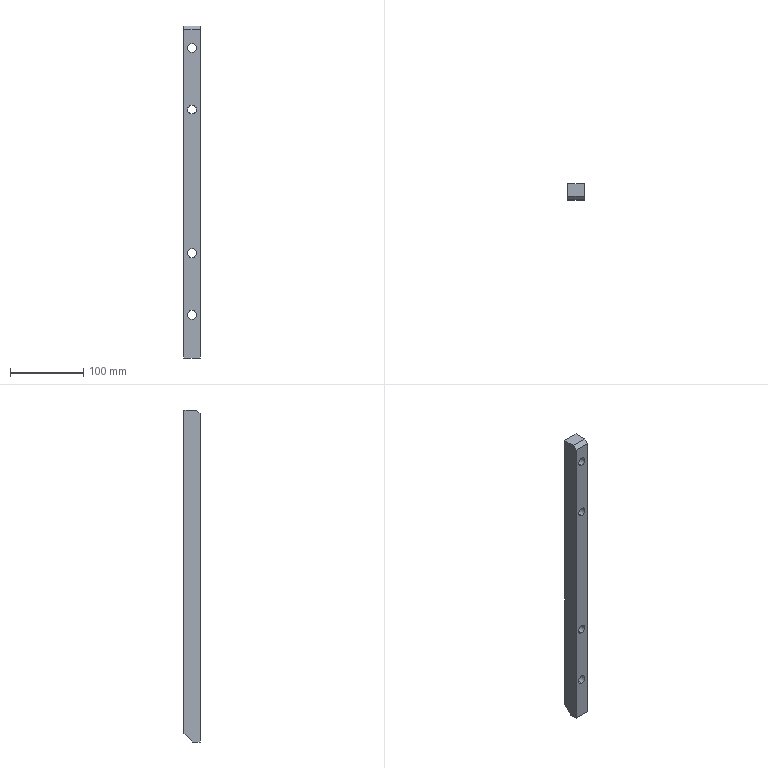Part | SolidWorks | features Chamfer 2, Extrusion 1, ICE 1 | 1 solid | 16 faces | box 22 x 22 x 453 mm | volume 207440 mm3 | cylinder 8 | plane 8 | commonest cylinder face diameters 12 x8
STEP:
#1=CARTESIAN_POINT('',(0.,-11.,190.5));
#2=VERTEX_POINT('',#1);
#3=CARTESIAN_POINT('',(0.,-11.,202.5));
#4=VERTEX_POINT('',#3);
#5=CARTESIAN_POINT('',(0.,-11.,196.5));
#6=DIRECTION('',(0.,1.,0.));
#7=DIRECTION('',(0.,0.,1.));
#8=AXIS2_PLACEMENT_3D('',#5,#6,#7);
#9=CIRCLE('',#8,6.);
#10=EDGE_CURVE('',#2,#4,#9,.T.);
#11=ORIENTED_EDGE('',*,*,#10,.F.);
#12=CARTESIAN_POINT('',(0.,11.,190.5));
#13=VERTEX_POINT('',#12);
#14=CARTESIAN_POINT('',(0.,-11.,190.5));
#15=DIRECTION('',(0.,1.,0.));
#16=VECTOR('',#15,1000.);
#17=LINE('',#14,#16);
#18=EDGE_CURVE('',#2,#13,#17,.T.);
#19=ORIENTED_EDGE('',*,*,#18,.T.);
#20=CARTESIAN_POINT('',(0.,11.,202.5));
#21=VERTEX_POINT('',#20);
#22=CARTESIAN_POINT('',(0.,11.,196.5));
#23=DIRECTION('',(0.,1.,0.));
#24=DIRECTION('',(0.,0.,1.));
#25=AXIS2_PLACEMENT_3D('',#22,#23,#24);
#26=CIRCLE('',#25,6.);
#27=EDGE_CURVE('',#13,#21,#26,.T.);
#28=ORIENTED_EDGE('',*,*,#27,.T.);
#29=CARTESIAN_POINT('',(0.,-11.,202.5));
#30=DIRECTION('',(0.,1.,0.));
#31=VECTOR('',#30,1000.);
#32=LINE('',#29,#31);
#33=EDGE_CURVE('',#4,#21,#32,.T.);
#34=ORIENTED_EDGE('',*,*,#33,.F.);
#35=EDGE_LOOP('',(#11,#19,#28,#34));
#36=FACE_OUTER_BOUND('',#35,.T.);
#37=CARTESIAN_POINT('',(0.,-11.,196.5));
#38=DIRECTION('',(0.,1.,0.));
#39=DIRECTION('',(0.,0.,1.));
#40=AXIS2_PLACEMENT_3D('',#37,#38,#39);
#41=CYLINDRICAL_SURFACE('',#40,6.);
#42=ADVANCED_FACE('',(#36),#41,.F.);
#43=CARTESIAN_POINT('',(0.,-11.,106.5));
#44=VERTEX_POINT('',#43);
#45=CARTESIAN_POINT('',(0.,-11.,118.5));
#46=VERTEX_POINT('',#45);
#47=CARTESIAN_POINT('',(0.,-11.,112.5));
#48=DIRECTION('',(0.,1.,0.));
#49=DIRECTION('',(0.,0.,1.));
#50=AXIS2_PLACEMENT_3D('',#47,#48,#49);
#51=CIRCLE('',#50,6.);
#52=EDGE_CURVE('',#44,#46,#51,.T.);
#53=ORIENTED_EDGE('',*,*,#52,.F.);
#54=CARTESIAN_POINT('',(0.,11.,106.5));
#55=VERTEX_POINT('',#54);
#56=CARTESIAN_POINT('',(0.,-11.,106.5));
#57=DIRECTION('',(0.,1.,0.));
#58=VECTOR('',#57,1000.);
#59=LINE('',#56,#58);
#60=EDGE_CURVE('',#44,#55,#59,.T.);
#61=ORIENTED_EDGE('',*,*,#60,.T.);
#62=CARTESIAN_POINT('',(0.,11.,118.5));
#63=VERTEX_POINT('',#62);
#64=CARTESIAN_POINT('',(0.,11.,112.5));
#65=DIRECTION('',(0.,1.,0.));
#66=DIRECTION('',(0.,0.,1.));
#67=AXIS2_PLACEMENT_3D('',#64,#65,#66);
#68=CIRCLE('',#67,6.);
#69=EDGE_CURVE('',#55,#63,#68,.T.);
#70=ORIENTED_EDGE('',*,*,#69,.T.);
#71=CARTESIAN_POINT('',(0.,-11.,118.5));
#72=DIRECTION('',(0.,1.,0.));
#73=VECTOR('',#72,1000.);
#74=LINE('',#71,#73);
#75=EDGE_CURVE('',#46,#63,#74,.T.);
#76=ORIENTED_EDGE('',*,*,#75,.F.);
#77=EDGE_LOOP('',(#53,#61,#70,#76));
#78=FACE_OUTER_BOUND('',#77,.T.);
#79=CARTESIAN_POINT('',(0.,-11.,112.5));
#80=DIRECTION('',(0.,1.,0.));
#81=DIRECTION('',(0.,0.,1.));
#82=AXIS2_PLACEMENT_3D('',#79,#80,#81);
#83=CYLINDRICAL_SURFACE('',#82,6.);
#84=ADVANCED_FACE('',(#78),#83,.F.);
#85=CARTESIAN_POINT('',(0.,-11.,-89.5));
#86=VERTEX_POINT('',#85);
#87=CARTESIAN_POINT('',(0.,-11.,-77.5));
#88=VERTEX_POINT('',#87);
#89=CARTESIAN_POINT('',(0.,-11.,-83.5));
#90=DIRECTION('',(0.,1.,0.));
#91=DIRECTION('',(0.,0.,1.));
#92=AXIS2_PLACEMENT_3D('',#89,#90,#91);
#93=CIRCLE('',#92,6.);
#94=EDGE_CURVE('',#86,#88,#93,.T.);
#95=ORIENTED_EDGE('',*,*,#94,.F.);
#96=CARTESIAN_POINT('',(0.,11.,-89.5));
#97=VERTEX_POINT('',#96);
#98=CARTESIAN_POINT('',(0.,-11.,-89.5));
#99=DIRECTION('',(0.,1.,0.));
#100=VECTOR('',#99,1000.);
#101=LINE('',#98,#100);
#102=EDGE_CURVE('',#86,#97,#101,.T.);
#103=ORIENTED_EDGE('',*,*,#102,.T.);
#104=CARTESIAN_POINT('',(0.,11.,-77.5));
#105=VERTEX_POINT('',#104);
#106=CARTESIAN_POINT('',(0.,11.,-83.5));
#107=DIRECTION('',(0.,1.,0.));
#108=DIRECTION('',(0.,0.,1.));
#109=AXIS2_PLACEMENT_3D('',#106,#107,#108);
#110=CIRCLE('',#109,6.);
#111=EDGE_CURVE('',#97,#105,#110,.T.);
#112=ORIENTED_EDGE('',*,*,#111,.T.);
#113=CARTESIAN_POINT('',(0.,-11.,-77.5));
#114=DIRECTION('',(0.,1.,0.));
#115=VECTOR('',#114,1000.);
#116=LINE('',#113,#115);
#117=EDGE_CURVE('',#88,#105,#116,.T.);
#118=ORIENTED_EDGE('',*,*,#117,.F.);
#119=EDGE_LOOP('',(#95,#103,#112,#118));
#120=FACE_OUTER_BOUND('',#119,.T.);
#121=CARTESIAN_POINT('',(0.,-11.,-83.5));
#122=DIRECTION('',(0.,1.,0.));
#123=DIRECTION('',(0.,0.,1.));
#124=AXIS2_PLACEMENT_3D('',#121,#122,#123);
#125=CYLINDRICAL_SURFACE('',#124,6.);
#126=ADVANCED_FACE('',(#120),#125,.F.);
#127=CARTESIAN_POINT('',(0.,-11.,-173.5));
#128=VERTEX_POINT('',#127);
#129=CARTESIAN_POINT('',(0.,-11.,-161.5));
#130=VERTEX_POINT('',#129);
#131=CARTESIAN_POINT('',(0.,-11.,-167.5));
#132=DIRECTION('',(0.,1.,0.));
#133=DIRECTION('',(0.,0.,1.));
#134=AXIS2_PLACEMENT_3D('',#131,#132,#133);
#135=CIRCLE('',#134,6.);
#136=EDGE_CURVE('',#128,#130,#135,.T.);
#137=ORIENTED_EDGE('',*,*,#136,.F.);
#138=CARTESIAN_POINT('',(0.,11.,-173.5));
#139=VERTEX_POINT('',#138);
#140=CARTESIAN_POINT('',(0.,-11.,-173.5));
#141=DIRECTION('',(0.,1.,0.));
#142=VECTOR('',#141,1000.);
#143=LINE('',#140,#142);
#144=EDGE_CURVE('',#128,#139,#143,.T.);
#145=ORIENTED_EDGE('',*,*,#144,.T.);
#146=CARTESIAN_POINT('',(0.,11.,-161.5));
#147=VERTEX_POINT('',#146);
#148=CARTESIAN_POINT('',(0.,11.,-167.5));
#149=DIRECTION('',(0.,1.,0.));
#150=DIRECTION('',(0.,0.,1.));
#151=AXIS2_PLACEMENT_3D('',#148,#149,#150);
#152=CIRCLE('',#151,6.);
#153=EDGE_CURVE('',#139,#147,#152,.T.);
#154=ORIENTED_EDGE('',*,*,#153,.T.);
#155=CARTESIAN_POINT('',(0.,-11.,-161.5));
#156=DIRECTION('',(0.,1.,0.));
#157=VECTOR('',#156,1000.);
#158=LINE('',#155,#157);
#159=EDGE_CURVE('',#130,#147,#158,.T.);
#160=ORIENTED_EDGE('',*,*,#159,.F.);
#161=EDGE_LOOP('',(#137,#145,#154,#160));
#162=FACE_OUTER_BOUND('',#161,.T.);
#163=CARTESIAN_POINT('',(0.,-11.,-167.5));
#164=DIRECTION('',(0.,1.,0.));
#165=DIRECTION('',(0.,0.,1.));
#166=AXIS2_PLACEMENT_3D('',#163,#164,#165);
#167=CYLINDRICAL_SURFACE('',#166,6.);
#168=ADVANCED_FACE('',(#162),#167,.F.);
#169=CARTESIAN_POINT('',(11.,-11.,-226.5));
#170=VERTEX_POINT('',#169);
#171=CARTESIAN_POINT('',(11.,-1.,-226.5));
#172=VERTEX_POINT('',#171);
#173=CARTESIAN_POINT('',(11.,11.,-226.5));
#174=DIRECTION('',(0.,1.,0.));
#175=VECTOR('',#174,1000.);
#176=LINE('',#173,#175);
#177=EDGE_CURVE('',#170,#172,#176,.T.);
#178=ORIENTED_EDGE('',*,*,#177,.T.);
#179=CARTESIAN_POINT('',(11.,11.,-214.5));
#180=VERTEX_POINT('',#179);
#181=CARTESIAN_POINT('',(11.,11.,-214.5));
#182=DIRECTION('',(0.,0.7071,0.7071));
#183=VECTOR('',#182,1000.);
#184=LINE('',#181,#183);
#185=EDGE_CURVE('',#172,#180,#184,.T.);
#186=ORIENTED_EDGE('',*,*,#185,.T.);
#187=CARTESIAN_POINT('',(11.,11.,226.5));
#188=VERTEX_POINT('',#187);
#189=CARTESIAN_POINT('',(11.,11.,226.5));
#190=DIRECTION('',(0.,0.,-1.));
#191=VECTOR('',#190,1000.);
#192=LINE('',#189,#191);
#193=EDGE_CURVE('',#188,#180,#192,.T.);
#194=ORIENTED_EDGE('',*,*,#193,.F.);
#195=CARTESIAN_POINT('',(11.,-6.,226.5));
#196=VERTEX_POINT('',#195);
#197=CARTESIAN_POINT('',(11.,11.,226.5));
#198=DIRECTION('',(0.,1.,0.));
#199=VECTOR('',#198,1000.);
#200=LINE('',#197,#199);
#201=EDGE_CURVE('',#196,#188,#200,.T.);
#202=ORIENTED_EDGE('',*,*,#201,.F.);
#203=CARTESIAN_POINT('',(11.,-11.,221.5));
#204=VERTEX_POINT('',#203);
#205=CARTESIAN_POINT('',(11.,-6.,226.5));
#206=DIRECTION('',(0.,-0.7071,-0.7071));
#207=VECTOR('',#206,1000.);
#208=LINE('',#205,#207);
#209=EDGE_CURVE('',#196,#204,#208,.T.);
#210=ORIENTED_EDGE('',*,*,#209,.T.);
#211=CARTESIAN_POINT('',(11.,-11.,226.5));
#212=DIRECTION('',(0.,0.,-1.));
#213=VECTOR('',#212,1000.);
#214=LINE('',#211,#213);
#215=EDGE_CURVE('',#204,#170,#214,.T.);
#216=ORIENTED_EDGE('',*,*,#215,.T.);
#217=EDGE_LOOP('',(#178,#186,#194,#202,#210,#216));
#218=FACE_OUTER_BOUND('',#217,.T.);
#219=CARTESIAN_POINT('',(11.,11.,226.5));
#220=DIRECTION('',(-1.,0.,0.));
#221=DIRECTION('',(0.,-1.,0.));
#222=AXIS2_PLACEMENT_3D('',#219,#220,#221);
#223=PLANE('',#222);
#224=ADVANCED_FACE('',(#218),#223,.F.);
#225=CARTESIAN_POINT('',(0.,11.,196.5));
#226=DIRECTION('',(0.,1.,0.));
#227=DIRECTION('',(0.,0.,1.));
#228=AXIS2_PLACEMENT_3D('',#225,#226,#227);
#229=CIRCLE('',#228,6.);
#230=EDGE_CURVE('',#21,#13,#229,.T.);
#231=ORIENTED_EDGE('',*,*,#230,.F.);
#232=ORIENTED_EDGE('',*,*,#27,.F.);
#233=EDGE_LOOP('',(#231,#232));
#234=FACE_BOUND('',#233,.T.);
#235=CARTESIAN_POINT('',(0.,11.,112.5));
#236=DIRECTION('',(0.,1.,0.));
#237=DIRECTION('',(0.,0.,1.));
#238=AXIS2_PLACEMENT_3D('',#235,#236,#237);
#239=CIRCLE('',#238,6.);
#240=EDGE_CURVE('',#63,#55,#239,.T.);
#241=ORIENTED_EDGE('',*,*,#240,.F.);
#242=ORIENTED_EDGE('',*,*,#69,.F.);
#243=EDGE_LOOP('',(#241,#242));
#244=FACE_BOUND('',#243,.T.);
#245=CARTESIAN_POINT('',(0.,11.,-83.5));
#246=DIRECTION('',(0.,1.,0.));
#247=DIRECTION('',(0.,0.,1.));
#248=AXIS2_PLACEMENT_3D('',#245,#246,#247);
#249=CIRCLE('',#248,6.);
#250=EDGE_CURVE('',#105,#97,#249,.T.);
#251=ORIENTED_EDGE('',*,*,#250,.F.);
#252=ORIENTED_EDGE('',*,*,#111,.F.);
#253=EDGE_LOOP('',(#251,#252));
#254=FACE_BOUND('',#253,.T.);
#255=CARTESIAN_POINT('',(0.,11.,-167.5));
#256=DIRECTION('',(0.,1.,0.));
#257=DIRECTION('',(0.,0.,1.));
#258=AXIS2_PLACEMENT_3D('',#255,#256,#257);
#259=CIRCLE('',#258,6.);
#260=EDGE_CURVE('',#147,#139,#259,.T.);
#261=ORIENTED_EDGE('',*,*,#260,.F.);
#262=ORIENTED_EDGE('',*,*,#153,.F.);
#263=EDGE_LOOP('',(#261,#262));
#264=FACE_BOUND('',#263,.T.);
#265=ORIENTED_EDGE('',*,*,#193,.T.);
#266=CARTESIAN_POINT('',(-11.,11.,-214.5));
#267=VERTEX_POINT('',#266);
#268=CARTESIAN_POINT('',(-11.,11.,-214.5));
#269=DIRECTION('',(-1.,0.,0.));
#270=VECTOR('',#269,1000.);
#271=LINE('',#268,#270);
#272=EDGE_CURVE('',#180,#267,#271,.T.);
#273=ORIENTED_EDGE('',*,*,#272,.T.);
#274=CARTESIAN_POINT('',(-11.,11.,226.5));
#275=VERTEX_POINT('',#274);
#276=CARTESIAN_POINT('',(-11.,11.,226.5));
#277=DIRECTION('',(0.,0.,-1.));
#278=VECTOR('',#277,1000.);
#279=LINE('',#276,#278);
#280=EDGE_CURVE('',#275,#267,#279,.T.);
#281=ORIENTED_EDGE('',*,*,#280,.F.);
#282=CARTESIAN_POINT('',(-11.,11.,226.5));
#283=DIRECTION('',(-1.,0.,0.));
#284=VECTOR('',#283,1000.);
#285=LINE('',#282,#284);
#286=EDGE_CURVE('',#188,#275,#285,.T.);
#287=ORIENTED_EDGE('',*,*,#286,.F.);
#288=EDGE_LOOP('',(#265,#273,#281,#287));
#289=FACE_OUTER_BOUND('',#288,.T.);
#290=CARTESIAN_POINT('',(-11.,11.,226.5));
#291=DIRECTION('',(0.,-1.,0.));
#292=DIRECTION('',(0.,0.,-1.));
#293=AXIS2_PLACEMENT_3D('',#290,#291,#292);
#294=PLANE('',#293);
#295=ADVANCED_FACE('',(#234,#244,#254,#264,#289),#294,.F.);
#296=ORIENTED_EDGE('',*,*,#280,.T.);
#297=CARTESIAN_POINT('',(-11.,-1.,-226.5));
#298=VERTEX_POINT('',#297);
#299=CARTESIAN_POINT('',(-11.,11.,-214.5));
#300=DIRECTION('',(0.,-0.7071,-0.7071));
#301=VECTOR('',#300,1000.);
#302=LINE('',#299,#301);
#303=EDGE_CURVE('',#267,#298,#302,.T.);
#304=ORIENTED_EDGE('',*,*,#303,.T.);
#305=CARTESIAN_POINT('',(-11.,-11.,-226.5));
#306=VERTEX_POINT('',#305);
#307=CARTESIAN_POINT('',(-11.,11.,-226.5));
#308=DIRECTION('',(0.,-1.,0.));
#309=VECTOR('',#308,1000.);
#310=LINE('',#307,#309);
#311=EDGE_CURVE('',#298,#306,#310,.T.);
#312=ORIENTED_EDGE('',*,*,#311,.T.);
#313=CARTESIAN_POINT('',(-11.,-11.,221.5));
#314=VERTEX_POINT('',#313);
#315=CARTESIAN_POINT('',(-11.,-11.,226.5));
#316=DIRECTION('',(0.,0.,-1.));
#317=VECTOR('',#316,1000.);
#318=LINE('',#315,#317);
#319=EDGE_CURVE('',#314,#306,#318,.T.);
#320=ORIENTED_EDGE('',*,*,#319,.F.);
#321=CARTESIAN_POINT('',(-11.,-6.,226.5));
#322=VERTEX_POINT('',#321);
#323=CARTESIAN_POINT('',(-11.,-6.,226.5));
#324=DIRECTION('',(0.,0.7071,0.7071));
#325=VECTOR('',#324,1000.);
#326=LINE('',#323,#325);
#327=EDGE_CURVE('',#314,#322,#326,.T.);
#328=ORIENTED_EDGE('',*,*,#327,.T.);
#329=CARTESIAN_POINT('',(-11.,11.,226.5));
#330=DIRECTION('',(0.,-1.,0.));
#331=VECTOR('',#330,1000.);
#332=LINE('',#329,#331);
#333=EDGE_CURVE('',#275,#322,#332,.T.);
#334=ORIENTED_EDGE('',*,*,#333,.F.);
#335=EDGE_LOOP('',(#296,#304,#312,#320,#328,#334));
#336=FACE_OUTER_BOUND('',#335,.T.);
#337=CARTESIAN_POINT('',(-11.,11.,226.5));
#338=DIRECTION('',(1.,0.,0.));
#339=DIRECTION('',(0.,1.,0.));
#340=AXIS2_PLACEMENT_3D('',#337,#338,#339);
#341=PLANE('',#340);
#342=ADVANCED_FACE('',(#336),#341,.F.);
#343=CARTESIAN_POINT('',(0.,-11.,196.5));
#344=DIRECTION('',(0.,1.,0.));
#345=DIRECTION('',(0.,0.,1.));
#346=AXIS2_PLACEMENT_3D('',#343,#344,#345);
#347=CIRCLE('',#346,6.);
#348=EDGE_CURVE('',#4,#2,#347,.T.);
#349=ORIENTED_EDGE('',*,*,#348,.T.);
#350=ORIENTED_EDGE('',*,*,#10,.T.);
#351=EDGE_LOOP('',(#349,#350));
#352=FACE_BOUND('',#351,.T.);
#353=CARTESIAN_POINT('',(0.,-11.,112.5));
#354=DIRECTION('',(0.,1.,0.));
#355=DIRECTION('',(0.,0.,1.));
#356=AXIS2_PLACEMENT_3D('',#353,#354,#355);
#357=CIRCLE('',#356,6.);
#358=EDGE_CURVE('',#46,#44,#357,.T.);
#359=ORIENTED_EDGE('',*,*,#358,.T.);
#360=ORIENTED_EDGE('',*,*,#52,.T.);
#361=EDGE_LOOP('',(#359,#360));
#362=FACE_BOUND('',#361,.T.);
#363=CARTESIAN_POINT('',(0.,-11.,-83.5));
#364=DIRECTION('',(0.,1.,0.));
#365=DIRECTION('',(0.,0.,1.));
#366=AXIS2_PLACEMENT_3D('',#363,#364,#365);
#367=CIRCLE('',#366,6.);
#368=EDGE_CURVE('',#88,#86,#367,.T.);
#369=ORIENTED_EDGE('',*,*,#368,.T.);
#370=ORIENTED_EDGE('',*,*,#94,.T.);
#371=EDGE_LOOP('',(#369,#370));
#372=FACE_BOUND('',#371,.T.);
#373=CARTESIAN_POINT('',(0.,-11.,-167.5));
#374=DIRECTION('',(0.,1.,0.));
#375=DIRECTION('',(0.,0.,1.));
#376=AXIS2_PLACEMENT_3D('',#373,#374,#375);
#377=CIRCLE('',#376,6.);
#378=EDGE_CURVE('',#130,#128,#377,.T.);
#379=ORIENTED_EDGE('',*,*,#378,.T.);
#380=ORIENTED_EDGE('',*,*,#136,.T.);
#381=EDGE_LOOP('',(#379,#380));
#382=FACE_BOUND('',#381,.T.);
#383=ORIENTED_EDGE('',*,*,#215,.F.);
#384=CARTESIAN_POINT('',(-11.,-11.,221.5));
#385=DIRECTION('',(-1.,0.,0.));
#386=VECTOR('',#385,1000.);
#387=LINE('',#384,#386);
#388=EDGE_CURVE('',#204,#314,#387,.T.);
#389=ORIENTED_EDGE('',*,*,#388,.T.);
#390=ORIENTED_EDGE('',*,*,#319,.T.);
#391=CARTESIAN_POINT('',(-11.,-11.,-226.5));
#392=DIRECTION('',(1.,0.,0.));
#393=VECTOR('',#392,1000.);
#394=LINE('',#391,#393);
#395=EDGE_CURVE('',#306,#170,#394,.T.);
#396=ORIENTED_EDGE('',*,*,#395,.T.);
#397=EDGE_LOOP('',(#383,#389,#390,#396));
#398=FACE_OUTER_BOUND('',#397,.T.);
#399=CARTESIAN_POINT('',(-11.,-11.,226.5));
#400=DIRECTION('',(0.,1.,0.));
#401=DIRECTION('',(0.,0.,1.));
#402=AXIS2_PLACEMENT_3D('',#399,#400,#401);
#403=PLANE('',#402);
#404=ADVANCED_FACE('',(#352,#362,#372,#382,#398),#403,.F.);
#405=ORIENTED_EDGE('',*,*,#333,.T.);
#406=CARTESIAN_POINT('',(11.,-6.,226.5));
#407=DIRECTION('',(1.,0.,0.));
#408=VECTOR('',#407,1000.);
#409=LINE('',#406,#408);
#410=EDGE_CURVE('',#322,#196,#409,.T.);
#411=ORIENTED_EDGE('',*,*,#410,.T.);
#412=ORIENTED_EDGE('',*,*,#201,.T.);
#413=ORIENTED_EDGE('',*,*,#286,.T.);
#414=EDGE_LOOP('',(#405,#411,#412,#413));
#415=FACE_OUTER_BOUND('',#414,.T.);
#416=CARTESIAN_POINT('',(0.,0.,226.5));
#417=DIRECTION('',(0.,0.,1.));
#418=DIRECTION('',(1.,0.,0.));
#419=AXIS2_PLACEMENT_3D('',#416,#417,#418);
#420=PLANE('',#419);
#421=ADVANCED_FACE('',(#415),#420,.T.);
#422=ORIENTED_EDGE('',*,*,#311,.F.);
#423=CARTESIAN_POINT('',(0.,-1.,-226.5));
#424=DIRECTION('',(1.,0.,0.));
#425=VECTOR('',#424,1000.);
#426=LINE('',#423,#425);
#427=EDGE_CURVE('',#298,#172,#426,.T.);
#428=ORIENTED_EDGE('',*,*,#427,.T.);
#429=ORIENTED_EDGE('',*,*,#177,.F.);
#430=ORIENTED_EDGE('',*,*,#395,.F.);
#431=EDGE_LOOP('',(#422,#428,#429,#430));
#432=FACE_OUTER_BOUND('',#431,.T.);
#433=CARTESIAN_POINT('',(0.,0.,-226.5));
#434=DIRECTION('',(0.,0.,1.));
#435=DIRECTION('',(1.,0.,0.));
#436=AXIS2_PLACEMENT_3D('',#433,#434,#435);
#437=PLANE('',#436);
#438=ADVANCED_FACE('',(#432),#437,.F.);
#439=ORIENTED_EDGE('',*,*,#144,.F.);
#440=ORIENTED_EDGE('',*,*,#378,.F.);
#441=ORIENTED_EDGE('',*,*,#159,.T.);
#442=ORIENTED_EDGE('',*,*,#260,.T.);
#443=EDGE_LOOP('',(#439,#440,#441,#442));
#444=FACE_OUTER_BOUND('',#443,.T.);
#445=CARTESIAN_POINT('',(0.,-11.,-167.5));
#446=DIRECTION('',(0.,1.,0.));
#447=DIRECTION('',(0.,0.,1.));
#448=AXIS2_PLACEMENT_3D('',#445,#446,#447);
#449=CYLINDRICAL_SURFACE('',#448,6.);
#450=ADVANCED_FACE('',(#444),#449,.F.);
#451=ORIENTED_EDGE('',*,*,#102,.F.);
#452=ORIENTED_EDGE('',*,*,#368,.F.);
#453=ORIENTED_EDGE('',*,*,#117,.T.);
#454=ORIENTED_EDGE('',*,*,#250,.T.);
#455=EDGE_LOOP('',(#451,#452,#453,#454));
#456=FACE_OUTER_BOUND('',#455,.T.);
#457=CARTESIAN_POINT('',(0.,-11.,-83.5));
#458=DIRECTION('',(0.,1.,0.));
#459=DIRECTION('',(0.,0.,1.));
#460=AXIS2_PLACEMENT_3D('',#457,#458,#459);
#461=CYLINDRICAL_SURFACE('',#460,6.);
#462=ADVANCED_FACE('',(#456),#461,.F.);
#463=ORIENTED_EDGE('',*,*,#60,.F.);
#464=ORIENTED_EDGE('',*,*,#358,.F.);
#465=ORIENTED_EDGE('',*,*,#75,.T.);
#466=ORIENTED_EDGE('',*,*,#240,.T.);
#467=EDGE_LOOP('',(#463,#464,#465,#466));
#468=FACE_OUTER_BOUND('',#467,.T.);
#469=CARTESIAN_POINT('',(0.,-11.,112.5));
#470=DIRECTION('',(0.,1.,0.));
#471=DIRECTION('',(0.,0.,1.));
#472=AXIS2_PLACEMENT_3D('',#469,#470,#471);
#473=CYLINDRICAL_SURFACE('',#472,6.);
#474=ADVANCED_FACE('',(#468),#473,.F.);
#475=ORIENTED_EDGE('',*,*,#18,.F.);
#476=ORIENTED_EDGE('',*,*,#348,.F.);
#477=ORIENTED_EDGE('',*,*,#33,.T.);
#478=ORIENTED_EDGE('',*,*,#230,.T.);
#479=EDGE_LOOP('',(#475,#476,#477,#478));
#480=FACE_OUTER_BOUND('',#479,.T.);
#481=CARTESIAN_POINT('',(0.,-11.,196.5));
#482=DIRECTION('',(0.,1.,0.));
#483=DIRECTION('',(0.,0.,1.));
#484=AXIS2_PLACEMENT_3D('',#481,#482,#483);
#485=CYLINDRICAL_SURFACE('',#484,6.);
#486=ADVANCED_FACE('',(#480),#485,.F.);
#487=ORIENTED_EDGE('',*,*,#327,.F.);
#488=ORIENTED_EDGE('',*,*,#388,.F.);
#489=ORIENTED_EDGE('',*,*,#209,.F.);
#490=ORIENTED_EDGE('',*,*,#410,.F.);
#491=EDGE_LOOP('',(#487,#488,#489,#490));
#492=FACE_OUTER_BOUND('',#491,.T.);
#493=CARTESIAN_POINT('',(0.,-6.,226.5));
#494=DIRECTION('',(0.,-0.7071,0.7071));
#495=DIRECTION('',(-1.,0.,0.));
#496=AXIS2_PLACEMENT_3D('',#493,#494,#495);
#497=PLANE('',#496);
#498=ADVANCED_FACE('',(#492),#497,.T.);
#499=ORIENTED_EDGE('',*,*,#185,.F.);
#500=ORIENTED_EDGE('',*,*,#427,.F.);
#501=ORIENTED_EDGE('',*,*,#303,.F.);
#502=ORIENTED_EDGE('',*,*,#272,.F.);
#503=EDGE_LOOP('',(#499,#500,#501,#502));
#504=FACE_OUTER_BOUND('',#503,.T.);
#505=CARTESIAN_POINT('',(-11.,11.,-214.5));
#506=DIRECTION('',(0.,-0.7071,0.7071));
#507=DIRECTION('',(-1.,0.,0.));
#508=AXIS2_PLACEMENT_3D('',#505,#506,#507);
#509=PLANE('',#508);
#510=ADVANCED_FACE('',(#504),#509,.F.);
#511=CLOSED_SHELL('',(#42,#84,#126,#168,#224,#295,#342,#404,#421,#438,#450,#462,#474,#486,#498,#510));
#512=MANIFOLD_SOLID_BREP('',#511);
#513=CARTESIAN_POINT('',(0.,0.,0.));
#514=DIRECTION('',(0.,0.,1.));
#515=DIRECTION('',(1.,0.,0.));
#516=AXIS2_PLACEMENT_3D('',#513,#514,#515);
#517=(LENGTH_UNIT()NAMED_UNIT(*)SI_UNIT(.MILLI.,.METRE.));
#518=UNCERTAINTY_MEASURE_WITH_UNIT(LENGTH_MEASURE(0.00001),#517,'','');
#519=(NAMED_UNIT(*)PLANE_ANGLE_UNIT()SI_UNIT($,.RADIAN.));
#520=(NAMED_UNIT(*)SI_UNIT($,.STERADIAN.)SOLID_ANGLE_UNIT());
#521=(GEOMETRIC_REPRESENTATION_CONTEXT(3)GLOBAL_UNCERTAINTY_ASSIGNED_CONTEXT((#518))GLOBAL_UNIT_ASSIGNED_CONTEXT((#517,#519,#520))REPRESENTATION_CONTEXT('',''));
#522=ADVANCED_BREP_SHAPE_REPRESENTATION('',(#512,#516),#521);